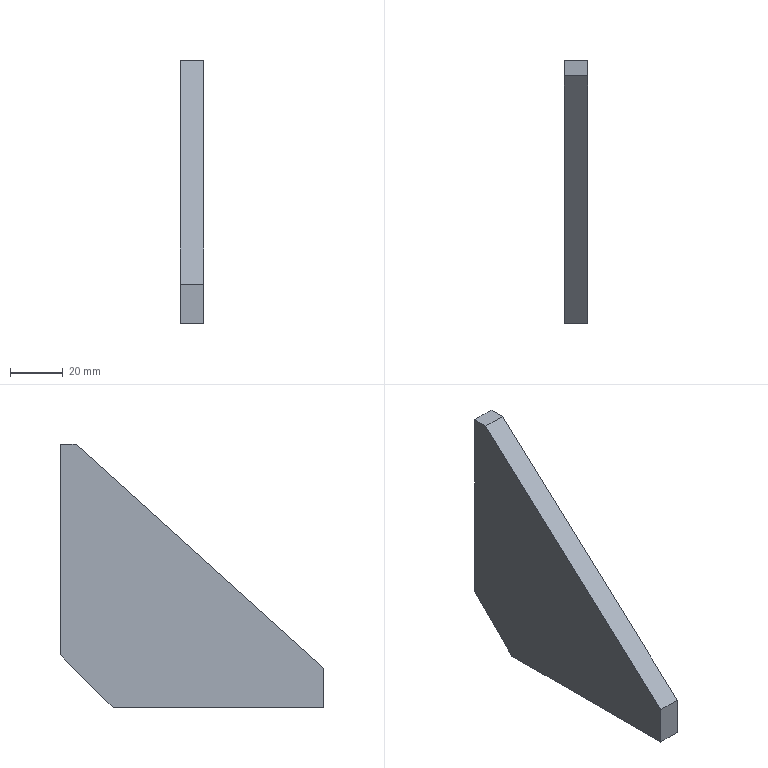Part | SolidWorks | features FlatPattern 1, SMBaseFlange 1, SheetMetal 1 | 1 solid | 8 faces | box 9 x 100 x 100 mm | volume 52245 mm3 | plane 8
STEP:
#1=CARTESIAN_POINT('',(0.,0.,0.));
#2=VERTEX_POINT('',#1);
#3=CARTESIAN_POINT('',(0.,-6.,0.));
#4=VERTEX_POINT('',#3);
#5=CARTESIAN_POINT('',(0.,-6.,0.));
#6=DIRECTION('',(0.,-1.,0.));
#7=VECTOR('',#6,1000.);
#8=LINE('',#5,#7);
#9=EDGE_CURVE('',#2,#4,#8,.T.);
#10=ORIENTED_EDGE('',*,*,#9,.F.);
#11=CARTESIAN_POINT('',(-9.,0.,0.));
#12=VERTEX_POINT('',#11);
#13=CARTESIAN_POINT('',(-9.,0.,0.));
#14=DIRECTION('',(1.,0.,0.));
#15=VECTOR('',#14,1000.);
#16=LINE('',#13,#15);
#17=EDGE_CURVE('',#12,#2,#16,.T.);
#18=ORIENTED_EDGE('',*,*,#17,.F.);
#19=CARTESIAN_POINT('',(-9.,-6.,0.));
#20=VERTEX_POINT('',#19);
#21=CARTESIAN_POINT('',(-9.,-6.,0.));
#22=DIRECTION('',(0.,-1.,0.));
#23=VECTOR('',#22,1000.);
#24=LINE('',#21,#23);
#25=EDGE_CURVE('',#12,#20,#24,.T.);
#26=ORIENTED_EDGE('',*,*,#25,.T.);
#27=CARTESIAN_POINT('',(-9.,-6.,0.));
#28=DIRECTION('',(1.,0.,0.));
#29=VECTOR('',#28,1000.);
#30=LINE('',#27,#29);
#31=EDGE_CURVE('',#20,#4,#30,.T.);
#32=ORIENTED_EDGE('',*,*,#31,.T.);
#33=EDGE_LOOP('',(#10,#18,#26,#32));
#34=FACE_OUTER_BOUND('',#33,.T.);
#35=CARTESIAN_POINT('',(-9.,-6.,0.));
#36=DIRECTION('',(0.,0.,1.));
#37=DIRECTION('',(1.,0.,0.));
#38=AXIS2_PLACEMENT_3D('',#35,#36,#37);
#39=PLANE('',#38);
#40=ADVANCED_FACE('',(#34),#39,.T.);
#41=CARTESIAN_POINT('',(0.,0.,-80.));
#42=VERTEX_POINT('',#41);
#43=CARTESIAN_POINT('',(0.,0.,0.));
#44=DIRECTION('',(0.,0.,1.));
#45=VECTOR('',#44,1000.);
#46=LINE('',#43,#45);
#47=EDGE_CURVE('',#42,#2,#46,.T.);
#48=ORIENTED_EDGE('',*,*,#47,.F.);
#49=CARTESIAN_POINT('',(-9.,0.,-80.));
#50=VERTEX_POINT('',#49);
#51=CARTESIAN_POINT('',(-9.,0.,-80.));
#52=DIRECTION('',(1.,0.,0.));
#53=VECTOR('',#52,1000.);
#54=LINE('',#51,#53);
#55=EDGE_CURVE('',#50,#42,#54,.T.);
#56=ORIENTED_EDGE('',*,*,#55,.F.);
#57=CARTESIAN_POINT('',(-9.,0.,0.));
#58=DIRECTION('',(0.,0.,1.));
#59=VECTOR('',#58,1000.);
#60=LINE('',#57,#59);
#61=EDGE_CURVE('',#50,#12,#60,.T.);
#62=ORIENTED_EDGE('',*,*,#61,.T.);
#63=ORIENTED_EDGE('',*,*,#17,.T.);
#64=EDGE_LOOP('',(#48,#56,#62,#63));
#65=FACE_OUTER_BOUND('',#64,.T.);
#66=CARTESIAN_POINT('',(-9.,0.,0.));
#67=DIRECTION('',(0.,1.,0.));
#68=DIRECTION('',(0.,0.,1.));
#69=AXIS2_PLACEMENT_3D('',#66,#67,#68);
#70=PLANE('',#69);
#71=ADVANCED_FACE('',(#65),#70,.T.);
#72=CARTESIAN_POINT('',(0.,-20.,-100.));
#73=VERTEX_POINT('',#72);
#74=CARTESIAN_POINT('',(0.,0.,-80.));
#75=DIRECTION('',(0.,0.7071,0.7071));
#76=VECTOR('',#75,1000.);
#77=LINE('',#74,#76);
#78=EDGE_CURVE('',#73,#42,#77,.T.);
#79=ORIENTED_EDGE('',*,*,#78,.F.);
#80=CARTESIAN_POINT('',(-9.,-20.,-100.));
#81=VERTEX_POINT('',#80);
#82=CARTESIAN_POINT('',(-9.,-20.,-100.));
#83=DIRECTION('',(1.,0.,0.));
#84=VECTOR('',#83,1000.);
#85=LINE('',#82,#84);
#86=EDGE_CURVE('',#81,#73,#85,.T.);
#87=ORIENTED_EDGE('',*,*,#86,.F.);
#88=CARTESIAN_POINT('',(-9.,0.,-80.));
#89=DIRECTION('',(0.,0.7071,0.7071));
#90=VECTOR('',#89,1000.);
#91=LINE('',#88,#90);
#92=EDGE_CURVE('',#81,#50,#91,.T.);
#93=ORIENTED_EDGE('',*,*,#92,.T.);
#94=ORIENTED_EDGE('',*,*,#55,.T.);
#95=EDGE_LOOP('',(#79,#87,#93,#94));
#96=FACE_OUTER_BOUND('',#95,.T.);
#97=CARTESIAN_POINT('',(-9.,0.,-80.));
#98=DIRECTION('',(0.,0.7071,-0.7071));
#99=DIRECTION('',(0.,0.7071,0.7071));
#100=AXIS2_PLACEMENT_3D('',#97,#98,#99);
#101=PLANE('',#100);
#102=ADVANCED_FACE('',(#96),#101,.T.);
#103=CARTESIAN_POINT('',(0.,-100.,-100.));
#104=VERTEX_POINT('',#103);
#105=CARTESIAN_POINT('',(0.,-20.,-100.));
#106=DIRECTION('',(0.,1.,0.));
#107=VECTOR('',#106,1000.);
#108=LINE('',#105,#107);
#109=EDGE_CURVE('',#104,#73,#108,.T.);
#110=ORIENTED_EDGE('',*,*,#109,.F.);
#111=CARTESIAN_POINT('',(-9.,-100.,-100.));
#112=VERTEX_POINT('',#111);
#113=CARTESIAN_POINT('',(-9.,-100.,-100.));
#114=DIRECTION('',(1.,0.,0.));
#115=VECTOR('',#114,1000.);
#116=LINE('',#113,#115);
#117=EDGE_CURVE('',#112,#104,#116,.T.);
#118=ORIENTED_EDGE('',*,*,#117,.F.);
#119=CARTESIAN_POINT('',(-9.,-20.,-100.));
#120=DIRECTION('',(0.,1.,0.));
#121=VECTOR('',#120,1000.);
#122=LINE('',#119,#121);
#123=EDGE_CURVE('',#112,#81,#122,.T.);
#124=ORIENTED_EDGE('',*,*,#123,.T.);
#125=ORIENTED_EDGE('',*,*,#86,.T.);
#126=EDGE_LOOP('',(#110,#118,#124,#125));
#127=FACE_OUTER_BOUND('',#126,.T.);
#128=CARTESIAN_POINT('',(-9.,-20.,-100.));
#129=DIRECTION('',(0.,0.,-1.));
#130=DIRECTION('',(0.,1.,0.));
#131=AXIS2_PLACEMENT_3D('',#128,#129,#130);
#132=PLANE('',#131);
#133=ADVANCED_FACE('',(#127),#132,.T.);
#134=CARTESIAN_POINT('',(0.,-100.,-85.));
#135=VERTEX_POINT('',#134);
#136=CARTESIAN_POINT('',(0.,-100.,-100.));
#137=DIRECTION('',(0.,0.,-1.));
#138=VECTOR('',#137,1000.);
#139=LINE('',#136,#138);
#140=EDGE_CURVE('',#135,#104,#139,.T.);
#141=ORIENTED_EDGE('',*,*,#140,.F.);
#142=CARTESIAN_POINT('',(-9.,-100.,-85.));
#143=VERTEX_POINT('',#142);
#144=CARTESIAN_POINT('',(-9.,-100.,-85.));
#145=DIRECTION('',(1.,0.,0.));
#146=VECTOR('',#145,1000.);
#147=LINE('',#144,#146);
#148=EDGE_CURVE('',#143,#135,#147,.T.);
#149=ORIENTED_EDGE('',*,*,#148,.F.);
#150=CARTESIAN_POINT('',(-9.,-100.,-100.));
#151=DIRECTION('',(0.,0.,-1.));
#152=VECTOR('',#151,1000.);
#153=LINE('',#150,#152);
#154=EDGE_CURVE('',#143,#112,#153,.T.);
#155=ORIENTED_EDGE('',*,*,#154,.T.);
#156=ORIENTED_EDGE('',*,*,#117,.T.);
#157=EDGE_LOOP('',(#141,#149,#155,#156));
#158=FACE_OUTER_BOUND('',#157,.T.);
#159=CARTESIAN_POINT('',(-9.,-100.,-100.));
#160=DIRECTION('',(0.,-1.,0.));
#161=DIRECTION('',(0.,0.,-1.));
#162=AXIS2_PLACEMENT_3D('',#159,#160,#161);
#163=PLANE('',#162);
#164=ADVANCED_FACE('',(#158),#163,.T.);
#165=CARTESIAN_POINT('',(0.,-100.,-85.));
#166=DIRECTION('',(0.,-0.7417,-0.6707));
#167=VECTOR('',#166,1000.);
#168=LINE('',#165,#167);
#169=EDGE_CURVE('',#4,#135,#168,.T.);
#170=ORIENTED_EDGE('',*,*,#169,.F.);
#171=ORIENTED_EDGE('',*,*,#31,.F.);
#172=CARTESIAN_POINT('',(-9.,-100.,-85.));
#173=DIRECTION('',(0.,-0.7417,-0.6707));
#174=VECTOR('',#173,1000.);
#175=LINE('',#172,#174);
#176=EDGE_CURVE('',#20,#143,#175,.T.);
#177=ORIENTED_EDGE('',*,*,#176,.T.);
#178=ORIENTED_EDGE('',*,*,#148,.T.);
#179=EDGE_LOOP('',(#170,#171,#177,#178));
#180=FACE_OUTER_BOUND('',#179,.T.);
#181=CARTESIAN_POINT('',(-9.,-100.,-85.));
#182=DIRECTION('',(0.,-0.6707,0.7417));
#183=DIRECTION('',(0.,-0.7417,-0.6707));
#184=AXIS2_PLACEMENT_3D('',#181,#182,#183);
#185=PLANE('',#184);
#186=ADVANCED_FACE('',(#180),#185,.T.);
#187=ORIENTED_EDGE('',*,*,#25,.F.);
#188=ORIENTED_EDGE('',*,*,#61,.F.);
#189=ORIENTED_EDGE('',*,*,#92,.F.);
#190=ORIENTED_EDGE('',*,*,#123,.F.);
#191=ORIENTED_EDGE('',*,*,#154,.F.);
#192=ORIENTED_EDGE('',*,*,#176,.F.);
#193=EDGE_LOOP('',(#187,#188,#189,#190,#191,#192));
#194=FACE_OUTER_BOUND('',#193,.T.);
#195=CARTESIAN_POINT('',(-9.,0.,0.));
#196=DIRECTION('',(-1.,0.,0.));
#197=DIRECTION('',(0.,0.,1.));
#198=AXIS2_PLACEMENT_3D('',#195,#196,#197);
#199=PLANE('',#198);
#200=ADVANCED_FACE('',(#194),#199,.T.);
#201=ORIENTED_EDGE('',*,*,#9,.T.);
#202=ORIENTED_EDGE('',*,*,#169,.T.);
#203=ORIENTED_EDGE('',*,*,#140,.T.);
#204=ORIENTED_EDGE('',*,*,#109,.T.);
#205=ORIENTED_EDGE('',*,*,#78,.T.);
#206=ORIENTED_EDGE('',*,*,#47,.T.);
#207=EDGE_LOOP('',(#201,#202,#203,#204,#205,#206));
#208=FACE_OUTER_BOUND('',#207,.T.);
#209=CARTESIAN_POINT('',(0.,0.,0.));
#210=DIRECTION('',(-1.,0.,0.));
#211=DIRECTION('',(0.,0.,1.));
#212=AXIS2_PLACEMENT_3D('',#209,#210,#211);
#213=PLANE('',#212);
#214=ADVANCED_FACE('',(#208),#213,.F.);
#215=CLOSED_SHELL('',(#40,#71,#102,#133,#164,#186,#200,#214));
#216=MANIFOLD_SOLID_BREP('',#215);
#217=CARTESIAN_POINT('',(0.,0.,0.));
#218=DIRECTION('',(0.,0.,1.));
#219=DIRECTION('',(1.,0.,0.));
#220=AXIS2_PLACEMENT_3D('',#217,#218,#219);
#221=(LENGTH_UNIT()NAMED_UNIT(*)SI_UNIT(.MILLI.,.METRE.));
#222=UNCERTAINTY_MEASURE_WITH_UNIT(LENGTH_MEASURE(0.00001),#221,'','');
#223=(NAMED_UNIT(*)PLANE_ANGLE_UNIT()SI_UNIT($,.RADIAN.));
#224=(NAMED_UNIT(*)SI_UNIT($,.STERADIAN.)SOLID_ANGLE_UNIT());
#225=(GEOMETRIC_REPRESENTATION_CONTEXT(3)GLOBAL_UNCERTAINTY_ASSIGNED_CONTEXT((#222))GLOBAL_UNIT_ASSIGNED_CONTEXT((#221,#223,#224))REPRESENTATION_CONTEXT('',''));
#226=ADVANCED_BREP_SHAPE_REPRESENTATION('',(#216,#220),#225);